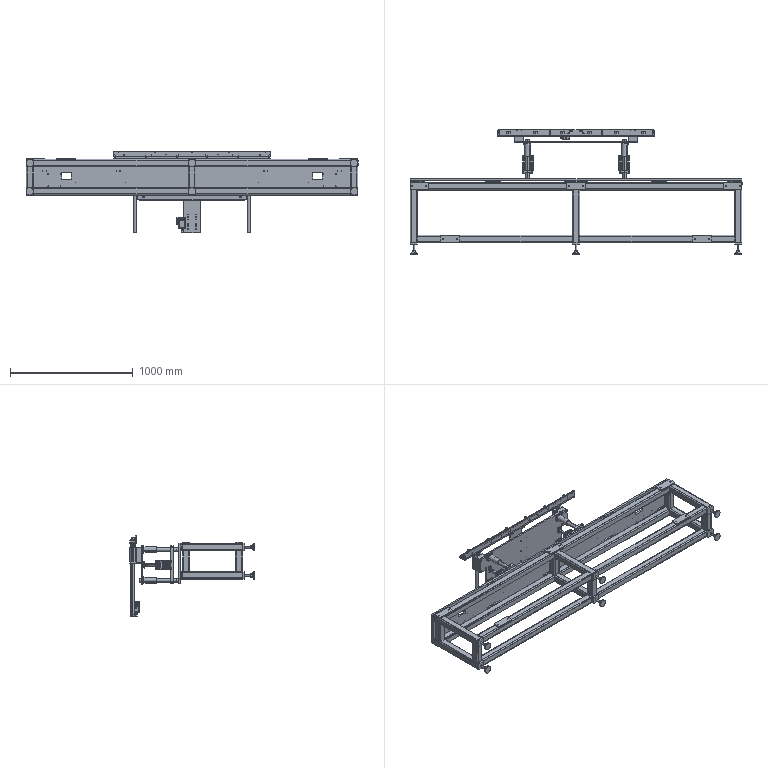Part | SolidWorks | features ReferencePattern 11, DerivedHolePattern 2, CompositeCurve 1 | 107 solids | 4996 faces | volume 39858660 mm3 | cylinder 2113 | plane 1821 | cone 680 | spline 344 | torus 38 | commonest cylinder face diameters 6.8 x152 10 x124 11 x124 6.6 x108 5 x106 3.3 x88